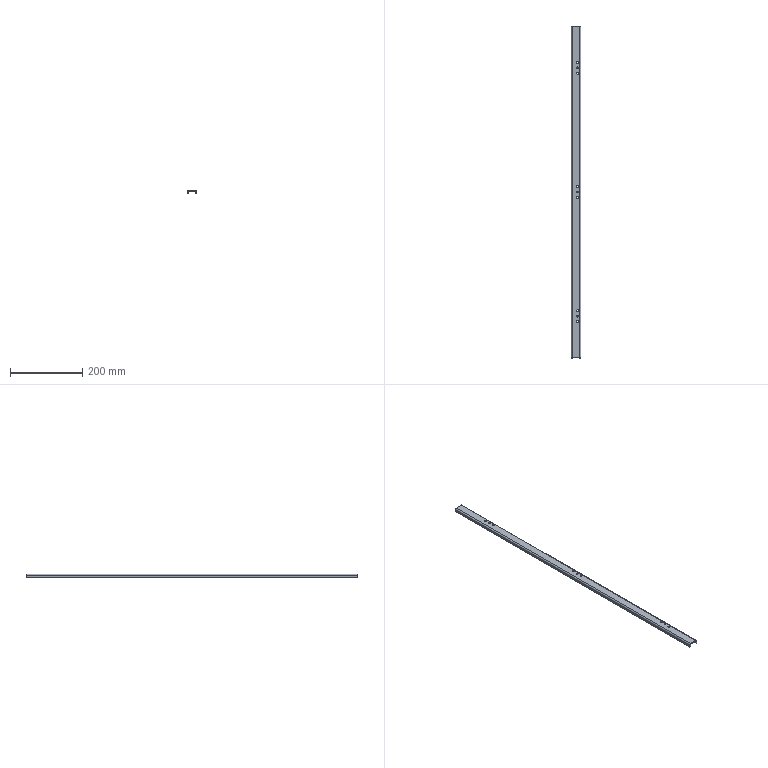Part | SolidWorks | features BaseBody 1 | 1 solid | 40 faces | box 27 x 919.8 x 10 mm | volume 107825 mm3 | cylinder 22 | plane 18 | commonest cylinder face diameters 5.2 x18 1 x2 7 x2
STEP:
#1=CARTESIAN_POINT('',(1.9,0.,-3.));
#2=VERTEX_POINT('',#1);
#3=CARTESIAN_POINT('',(1.9,0.,0.));
#4=VERTEX_POINT('',#3);
#5=CARTESIAN_POINT('',(1.9,0.,-3.));
#6=DIRECTION('',(0.,0.,1.));
#7=VECTOR('',#6,1000.);
#8=LINE('',#5,#7);
#9=EDGE_CURVE('',#2,#4,#8,.T.);
#10=ORIENTED_EDGE('',*,*,#9,.F.);
#11=CARTESIAN_POINT('',(7.1,0.,-3.));
#12=VERTEX_POINT('',#11);
#13=CARTESIAN_POINT('',(4.5,0.,-3.));
#14=DIRECTION('',(0.,0.,1.));
#15=DIRECTION('',(1.,0.,0.));
#16=AXIS2_PLACEMENT_3D('',#13,#14,#15);
#17=CIRCLE('',#16,2.6);
#18=EDGE_CURVE('',#12,#2,#17,.T.);
#19=ORIENTED_EDGE('',*,*,#18,.F.);
#20=CARTESIAN_POINT('',(7.1,0.,0.));
#21=VERTEX_POINT('',#20);
#22=CARTESIAN_POINT('',(7.1,0.,-3.));
#23=DIRECTION('',(0.,0.,1.));
#24=VECTOR('',#23,1000.);
#25=LINE('',#22,#24);
#26=EDGE_CURVE('',#12,#21,#25,.T.);
#27=ORIENTED_EDGE('',*,*,#26,.T.);
#28=CARTESIAN_POINT('',(4.5,0.,0.));
#29=DIRECTION('',(0.,0.,1.));
#30=DIRECTION('',(1.,0.,0.));
#31=AXIS2_PLACEMENT_3D('',#28,#29,#30);
#32=CIRCLE('',#31,2.6);
#33=EDGE_CURVE('',#21,#4,#32,.T.);
#34=ORIENTED_EDGE('',*,*,#33,.T.);
#35=EDGE_LOOP('',(#10,#19,#27,#34));
#36=FACE_OUTER_BOUND('',#35,.T.);
#37=CARTESIAN_POINT('',(4.5,0.,-3.));
#38=DIRECTION('',(0.,0.,1.));
#39=DIRECTION('',(1.,0.,0.));
#40=AXIS2_PLACEMENT_3D('',#37,#38,#39);
#41=CYLINDRICAL_SURFACE('',#40,2.6);
#42=ADVANCED_FACE('',(#36),#41,.F.);
#43=CARTESIAN_POINT('',(1.9,15.,-3.));
#44=VERTEX_POINT('',#43);
#45=CARTESIAN_POINT('',(1.9,15.,0.));
#46=VERTEX_POINT('',#45);
#47=CARTESIAN_POINT('',(1.9,15.,-3.));
#48=DIRECTION('',(0.,0.,1.));
#49=VECTOR('',#48,1000.);
#50=LINE('',#47,#49);
#51=EDGE_CURVE('',#44,#46,#50,.T.);
#52=ORIENTED_EDGE('',*,*,#51,.F.);
#53=CARTESIAN_POINT('',(7.1,15.,-3.));
#54=VERTEX_POINT('',#53);
#55=CARTESIAN_POINT('',(4.5,15.,-3.));
#56=DIRECTION('',(0.,0.,1.));
#57=DIRECTION('',(1.,0.,0.));
#58=AXIS2_PLACEMENT_3D('',#55,#56,#57);
#59=CIRCLE('',#58,2.6);
#60=EDGE_CURVE('',#54,#44,#59,.T.);
#61=ORIENTED_EDGE('',*,*,#60,.F.);
#62=CARTESIAN_POINT('',(7.1,15.,0.));
#63=VERTEX_POINT('',#62);
#64=CARTESIAN_POINT('',(7.1,15.,-3.));
#65=DIRECTION('',(0.,0.,1.));
#66=VECTOR('',#65,1000.);
#67=LINE('',#64,#66);
#68=EDGE_CURVE('',#54,#63,#67,.T.);
#69=ORIENTED_EDGE('',*,*,#68,.T.);
#70=CARTESIAN_POINT('',(4.5,15.,0.));
#71=DIRECTION('',(0.,0.,1.));
#72=DIRECTION('',(1.,0.,0.));
#73=AXIS2_PLACEMENT_3D('',#70,#71,#72);
#74=CIRCLE('',#73,2.6);
#75=EDGE_CURVE('',#63,#46,#74,.T.);
#76=ORIENTED_EDGE('',*,*,#75,.T.);
#77=EDGE_LOOP('',(#52,#61,#69,#76));
#78=FACE_OUTER_BOUND('',#77,.T.);
#79=CARTESIAN_POINT('',(4.5,15.,-3.));
#80=DIRECTION('',(0.,0.,1.));
#81=DIRECTION('',(1.,0.,0.));
#82=AXIS2_PLACEMENT_3D('',#79,#80,#81);
#83=CYLINDRICAL_SURFACE('',#82,2.6);
#84=ADVANCED_FACE('',(#78),#83,.F.);
#85=CARTESIAN_POINT('',(1.9,-15.,-3.));
#86=VERTEX_POINT('',#85);
#87=CARTESIAN_POINT('',(1.9,-15.,0.));
#88=VERTEX_POINT('',#87);
#89=CARTESIAN_POINT('',(1.9,-15.,-3.));
#90=DIRECTION('',(0.,0.,1.));
#91=VECTOR('',#90,1000.);
#92=LINE('',#89,#91);
#93=EDGE_CURVE('',#86,#88,#92,.T.);
#94=ORIENTED_EDGE('',*,*,#93,.F.);
#95=CARTESIAN_POINT('',(7.1,-15.,-3.));
#96=VERTEX_POINT('',#95);
#97=CARTESIAN_POINT('',(4.5,-15.,-3.));
#98=DIRECTION('',(0.,0.,1.));
#99=DIRECTION('',(1.,0.,0.));
#100=AXIS2_PLACEMENT_3D('',#97,#98,#99);
#101=CIRCLE('',#100,2.6);
#102=EDGE_CURVE('',#96,#86,#101,.T.);
#103=ORIENTED_EDGE('',*,*,#102,.F.);
#104=CARTESIAN_POINT('',(7.1,-15.,0.));
#105=VERTEX_POINT('',#104);
#106=CARTESIAN_POINT('',(7.1,-15.,-3.));
#107=DIRECTION('',(0.,0.,1.));
#108=VECTOR('',#107,1000.);
#109=LINE('',#106,#108);
#110=EDGE_CURVE('',#96,#105,#109,.T.);
#111=ORIENTED_EDGE('',*,*,#110,.T.);
#112=CARTESIAN_POINT('',(4.5,-15.,0.));
#113=DIRECTION('',(0.,0.,1.));
#114=DIRECTION('',(1.,0.,0.));
#115=AXIS2_PLACEMENT_3D('',#112,#113,#114);
#116=CIRCLE('',#115,2.6);
#117=EDGE_CURVE('',#105,#88,#116,.T.);
#118=ORIENTED_EDGE('',*,*,#117,.T.);
#119=EDGE_LOOP('',(#94,#103,#111,#118));
#120=FACE_OUTER_BOUND('',#119,.T.);
#121=CARTESIAN_POINT('',(4.5,-15.,-3.));
#122=DIRECTION('',(0.,0.,1.));
#123=DIRECTION('',(1.,0.,0.));
#124=AXIS2_PLACEMENT_3D('',#121,#122,#123);
#125=CYLINDRICAL_SURFACE('',#124,2.6);
#126=ADVANCED_FACE('',(#120),#125,.F.);
#127=CARTESIAN_POINT('',(1.9,-359.,-3.));
#128=VERTEX_POINT('',#127);
#129=CARTESIAN_POINT('',(1.9,-359.,0.));
#130=VERTEX_POINT('',#129);
#131=CARTESIAN_POINT('',(1.9,-359.,-3.));
#132=DIRECTION('',(0.,0.,1.));
#133=VECTOR('',#132,1000.);
#134=LINE('',#131,#133);
#135=EDGE_CURVE('',#128,#130,#134,.T.);
#136=ORIENTED_EDGE('',*,*,#135,.F.);
#137=CARTESIAN_POINT('',(7.1,-359.,-3.));
#138=VERTEX_POINT('',#137);
#139=CARTESIAN_POINT('',(4.5,-359.,-3.));
#140=DIRECTION('',(0.,0.,1.));
#141=DIRECTION('',(1.,0.,0.));
#142=AXIS2_PLACEMENT_3D('',#139,#140,#141);
#143=CIRCLE('',#142,2.6);
#144=EDGE_CURVE('',#138,#128,#143,.T.);
#145=ORIENTED_EDGE('',*,*,#144,.F.);
#146=CARTESIAN_POINT('',(7.1,-359.,0.));
#147=VERTEX_POINT('',#146);
#148=CARTESIAN_POINT('',(7.1,-359.,-3.));
#149=DIRECTION('',(0.,0.,1.));
#150=VECTOR('',#149,1000.);
#151=LINE('',#148,#150);
#152=EDGE_CURVE('',#138,#147,#151,.T.);
#153=ORIENTED_EDGE('',*,*,#152,.T.);
#154=CARTESIAN_POINT('',(4.5,-359.,0.));
#155=DIRECTION('',(0.,0.,1.));
#156=DIRECTION('',(1.,0.,0.));
#157=AXIS2_PLACEMENT_3D('',#154,#155,#156);
#158=CIRCLE('',#157,2.6);
#159=EDGE_CURVE('',#147,#130,#158,.T.);
#160=ORIENTED_EDGE('',*,*,#159,.T.);
#161=EDGE_LOOP('',(#136,#145,#153,#160));
#162=FACE_OUTER_BOUND('',#161,.T.);
#163=CARTESIAN_POINT('',(4.5,-359.,-3.));
#164=DIRECTION('',(0.,0.,1.));
#165=DIRECTION('',(1.,0.,0.));
#166=AXIS2_PLACEMENT_3D('',#163,#164,#165);
#167=CYLINDRICAL_SURFACE('',#166,2.6);
#168=ADVANCED_FACE('',(#162),#167,.F.);
#169=CARTESIAN_POINT('',(1.9,-344.,-3.));
#170=VERTEX_POINT('',#169);
#171=CARTESIAN_POINT('',(1.9,-344.,0.));
#172=VERTEX_POINT('',#171);
#173=CARTESIAN_POINT('',(1.9,-344.,-3.));
#174=DIRECTION('',(0.,0.,1.));
#175=VECTOR('',#174,1000.);
#176=LINE('',#173,#175);
#177=EDGE_CURVE('',#170,#172,#176,.T.);
#178=ORIENTED_EDGE('',*,*,#177,.F.);
#179=CARTESIAN_POINT('',(7.1,-344.,-3.));
#180=VERTEX_POINT('',#179);
#181=CARTESIAN_POINT('',(4.5,-344.,-3.));
#182=DIRECTION('',(0.,0.,1.));
#183=DIRECTION('',(1.,0.,0.));
#184=AXIS2_PLACEMENT_3D('',#181,#182,#183);
#185=CIRCLE('',#184,2.6);
#186=EDGE_CURVE('',#180,#170,#185,.T.);
#187=ORIENTED_EDGE('',*,*,#186,.F.);
#188=CARTESIAN_POINT('',(7.1,-344.,0.));
#189=VERTEX_POINT('',#188);
#190=CARTESIAN_POINT('',(7.1,-344.,-3.));
#191=DIRECTION('',(0.,0.,1.));
#192=VECTOR('',#191,1000.);
#193=LINE('',#190,#192);
#194=EDGE_CURVE('',#180,#189,#193,.T.);
#195=ORIENTED_EDGE('',*,*,#194,.T.);
#196=CARTESIAN_POINT('',(4.5,-344.,0.));
#197=DIRECTION('',(0.,0.,1.));
#198=DIRECTION('',(1.,0.,0.));
#199=AXIS2_PLACEMENT_3D('',#196,#197,#198);
#200=CIRCLE('',#199,2.6);
#201=EDGE_CURVE('',#189,#172,#200,.T.);
#202=ORIENTED_EDGE('',*,*,#201,.T.);
#203=EDGE_LOOP('',(#178,#187,#195,#202));
#204=FACE_OUTER_BOUND('',#203,.T.);
#205=CARTESIAN_POINT('',(4.5,-344.,-3.));
#206=DIRECTION('',(0.,0.,1.));
#207=DIRECTION('',(1.,0.,0.));
#208=AXIS2_PLACEMENT_3D('',#205,#206,#207);
#209=CYLINDRICAL_SURFACE('',#208,2.6);
#210=ADVANCED_FACE('',(#204),#209,.F.);
#211=CARTESIAN_POINT('',(1.9,-329.,-3.));
#212=VERTEX_POINT('',#211);
#213=CARTESIAN_POINT('',(1.9,-329.,0.));
#214=VERTEX_POINT('',#213);
#215=CARTESIAN_POINT('',(1.9,-329.,-3.));
#216=DIRECTION('',(0.,0.,1.));
#217=VECTOR('',#216,1000.);
#218=LINE('',#215,#217);
#219=EDGE_CURVE('',#212,#214,#218,.T.);
#220=ORIENTED_EDGE('',*,*,#219,.F.);
#221=CARTESIAN_POINT('',(7.1,-329.,-3.));
#222=VERTEX_POINT('',#221);
#223=CARTESIAN_POINT('',(4.5,-329.,-3.));
#224=DIRECTION('',(0.,0.,1.));
#225=DIRECTION('',(1.,0.,0.));
#226=AXIS2_PLACEMENT_3D('',#223,#224,#225);
#227=CIRCLE('',#226,2.6);
#228=EDGE_CURVE('',#222,#212,#227,.T.);
#229=ORIENTED_EDGE('',*,*,#228,.F.);
#230=CARTESIAN_POINT('',(7.1,-329.,0.));
#231=VERTEX_POINT('',#230);
#232=CARTESIAN_POINT('',(7.1,-329.,-3.));
#233=DIRECTION('',(0.,0.,1.));
#234=VECTOR('',#233,1000.);
#235=LINE('',#232,#234);
#236=EDGE_CURVE('',#222,#231,#235,.T.);
#237=ORIENTED_EDGE('',*,*,#236,.T.);
#238=CARTESIAN_POINT('',(4.5,-329.,0.));
#239=DIRECTION('',(0.,0.,1.));
#240=DIRECTION('',(1.,0.,0.));
#241=AXIS2_PLACEMENT_3D('',#238,#239,#240);
#242=CIRCLE('',#241,2.6);
#243=EDGE_CURVE('',#231,#214,#242,.T.);
#244=ORIENTED_EDGE('',*,*,#243,.T.);
#245=EDGE_LOOP('',(#220,#229,#237,#244));
#246=FACE_OUTER_BOUND('',#245,.T.);
#247=CARTESIAN_POINT('',(4.5,-329.,-3.));
#248=DIRECTION('',(0.,0.,1.));
#249=DIRECTION('',(1.,0.,0.));
#250=AXIS2_PLACEMENT_3D('',#247,#248,#249);
#251=CYLINDRICAL_SURFACE('',#250,2.6);
#252=ADVANCED_FACE('',(#246),#251,.F.);
#253=CARTESIAN_POINT('',(-10.5,459.9,-10.));
#254=VERTEX_POINT('',#253);
#255=CARTESIAN_POINT('',(-10.5,-459.9,-10.));
#256=VERTEX_POINT('',#255);
#257=CARTESIAN_POINT('',(-10.5,-459.9,-10.));
#258=DIRECTION('',(0.,-1.,0.));
#259=VECTOR('',#258,1000.);
#260=LINE('',#257,#259);
#261=EDGE_CURVE('',#254,#256,#260,.T.);
#262=ORIENTED_EDGE('',*,*,#261,.T.);
#263=CARTESIAN_POINT('',(-13.5,-459.9,-10.));
#264=VERTEX_POINT('',#263);
#265=CARTESIAN_POINT('',(-13.5,-459.9,-10.));
#266=DIRECTION('',(1.,0.,0.));
#267=VECTOR('',#266,1000.);
#268=LINE('',#265,#267);
#269=EDGE_CURVE('',#264,#256,#268,.T.);
#270=ORIENTED_EDGE('',*,*,#269,.F.);
#271=CARTESIAN_POINT('',(-13.5,459.9,-10.));
#272=VERTEX_POINT('',#271);
#273=CARTESIAN_POINT('',(-13.5,0.,-10.));
#274=DIRECTION('',(0.,-1.,0.));
#275=VECTOR('',#274,1000.);
#276=LINE('',#273,#275);
#277=EDGE_CURVE('',#272,#264,#276,.T.);
#278=ORIENTED_EDGE('',*,*,#277,.F.);
#279=CARTESIAN_POINT('',(-13.5,459.9,-10.));
#280=DIRECTION('',(1.,0.,0.));
#281=VECTOR('',#280,1000.);
#282=LINE('',#279,#281);
#283=EDGE_CURVE('',#272,#254,#282,.T.);
#284=ORIENTED_EDGE('',*,*,#283,.T.);
#285=EDGE_LOOP('',(#262,#270,#278,#284));
#286=FACE_OUTER_BOUND('',#285,.T.);
#287=CARTESIAN_POINT('',(-13.5,-459.9,-10.));
#288=DIRECTION('',(0.,0.,1.));
#289=DIRECTION('',(1.,0.,0.));
#290=AXIS2_PLACEMENT_3D('',#287,#288,#289);
#291=PLANE('',#290);
#292=ADVANCED_FACE('',(#286),#291,.F.);
#293=CARTESIAN_POINT('',(-10.5,459.9,-3.5));
#294=VERTEX_POINT('',#293);
#295=CARTESIAN_POINT('',(-10.5,459.9,-10.));
#296=DIRECTION('',(0.,0.,-1.));
#297=VECTOR('',#296,1000.);
#298=LINE('',#295,#297);
#299=EDGE_CURVE('',#294,#254,#298,.T.);
#300=ORIENTED_EDGE('',*,*,#299,.F.);
#301=CARTESIAN_POINT('',(-10.5,-459.9,-3.5));
#302=VERTEX_POINT('',#301);
#303=CARTESIAN_POINT('',(-10.5,-459.9,-3.5));
#304=DIRECTION('',(0.,1.,0.));
#305=VECTOR('',#304,1000.);
#306=LINE('',#303,#305);
#307=EDGE_CURVE('',#302,#294,#306,.T.);
#308=ORIENTED_EDGE('',*,*,#307,.F.);
#309=CARTESIAN_POINT('',(-10.5,-459.9,-3.));
#310=DIRECTION('',(0.,0.,1.));
#311=VECTOR('',#310,1000.);
#312=LINE('',#309,#311);
#313=EDGE_CURVE('',#256,#302,#312,.T.);
#314=ORIENTED_EDGE('',*,*,#313,.F.);
#315=ORIENTED_EDGE('',*,*,#261,.F.);
#316=EDGE_LOOP('',(#300,#308,#314,#315));
#317=FACE_OUTER_BOUND('',#316,.T.);
#318=CARTESIAN_POINT('',(-10.5,0.,0.));
#319=DIRECTION('',(1.,0.,0.));
#320=DIRECTION('',(0.,0.,-1.));
#321=AXIS2_PLACEMENT_3D('',#318,#319,#320);
#322=PLANE('',#321);
#323=ADVANCED_FACE('',(#317),#322,.T.);
#324=CARTESIAN_POINT('',(-13.5,459.9,-3.5));
#325=VERTEX_POINT('',#324);
#326=CARTESIAN_POINT('',(-13.5,-459.9,-3.5));
#327=VERTEX_POINT('',#326);
#328=CARTESIAN_POINT('',(-13.5,-459.9,-3.5));
#329=DIRECTION('',(0.,-1.,0.));
#330=VECTOR('',#329,1000.);
#331=LINE('',#328,#330);
#332=EDGE_CURVE('',#325,#327,#331,.T.);
#333=ORIENTED_EDGE('',*,*,#332,.F.);
#334=CARTESIAN_POINT('',(-13.5,459.9,0.));
#335=DIRECTION('',(0.,0.,-1.));
#336=VECTOR('',#335,1000.);
#337=LINE('',#334,#336);
#338=EDGE_CURVE('',#325,#272,#337,.T.);
#339=ORIENTED_EDGE('',*,*,#338,.T.);
#340=ORIENTED_EDGE('',*,*,#277,.T.);
#341=CARTESIAN_POINT('',(-13.5,-459.9,0.));
#342=DIRECTION('',(0.,0.,1.));
#343=VECTOR('',#342,1000.);
#344=LINE('',#341,#343);
#345=EDGE_CURVE('',#264,#327,#344,.T.);
#346=ORIENTED_EDGE('',*,*,#345,.T.);
#347=EDGE_LOOP('',(#333,#339,#340,#346));
#348=FACE_OUTER_BOUND('',#347,.T.);
#349=CARTESIAN_POINT('',(-13.5,0.,0.));
#350=DIRECTION('',(1.,0.,0.));
#351=DIRECTION('',(0.,0.,-1.));
#352=AXIS2_PLACEMENT_3D('',#349,#350,#351);
#353=PLANE('',#352);
#354=ADVANCED_FACE('',(#348),#353,.F.);
#355=CARTESIAN_POINT('',(-13.5,-459.9,-3.5));
#356=DIRECTION('',(-1.,0.,0.));
#357=VECTOR('',#356,1000.);
#358=LINE('',#355,#357);
#359=EDGE_CURVE('',#302,#327,#358,.T.);
#360=ORIENTED_EDGE('',*,*,#359,.T.);
#361=ORIENTED_EDGE('',*,*,#345,.F.);
#362=ORIENTED_EDGE('',*,*,#269,.T.);
#363=ORIENTED_EDGE('',*,*,#313,.T.);
#364=EDGE_LOOP('',(#360,#361,#362,#363));
#365=FACE_OUTER_BOUND('',#364,.T.);
#366=CARTESIAN_POINT('',(-13.5,-459.9,-3.));
#367=DIRECTION('',(0.,1.,0.));
#368=DIRECTION('',(1.,0.,0.));
#369=AXIS2_PLACEMENT_3D('',#366,#367,#368);
#370=PLANE('',#369);
#371=ADVANCED_FACE('',(#365),#370,.F.);
#372=CARTESIAN_POINT('',(-10.5,459.9,-3.5));
#373=DIRECTION('',(-1.,0.,0.));
#374=VECTOR('',#373,1000.);
#375=LINE('',#372,#374);
#376=EDGE_CURVE('',#294,#325,#375,.T.);
#377=ORIENTED_EDGE('',*,*,#376,.F.);
#378=ORIENTED_EDGE('',*,*,#299,.T.);
#379=ORIENTED_EDGE('',*,*,#283,.F.);
#380=ORIENTED_EDGE('',*,*,#338,.F.);
#381=EDGE_LOOP('',(#377,#378,#379,#380));
#382=FACE_OUTER_BOUND('',#381,.T.);
#383=CARTESIAN_POINT('',(-13.5,459.9,-10.));
#384=DIRECTION('',(0.,-1.,0.));
#385=DIRECTION('',(0.,0.,-1.));
#386=AXIS2_PLACEMENT_3D('',#383,#384,#385);
#387=PLANE('',#386);
#388=ADVANCED_FACE('',(#382),#387,.F.);
#389=CARTESIAN_POINT('',(-10.,459.9,-3.));
#390=VERTEX_POINT('',#389);
#391=CARTESIAN_POINT('',(-10.,-459.9,-3.));
#392=VERTEX_POINT('',#391);
#393=CARTESIAN_POINT('',(-10.,459.9,-3.));
#394=DIRECTION('',(0.,-1.,0.));
#395=VECTOR('',#394,1000.);
#396=LINE('',#393,#395);
#397=EDGE_CURVE('',#390,#392,#396,.T.);
#398=ORIENTED_EDGE('',*,*,#397,.T.);
#399=CARTESIAN_POINT('',(-10.,-459.9,-3.5));
#400=DIRECTION('',(0.,-1.,0.));
#401=DIRECTION('',(0.,0.,1.));
#402=AXIS2_PLACEMENT_3D('',#399,#400,#401);
#403=CIRCLE('',#402,0.5);
#404=EDGE_CURVE('',#392,#302,#403,.T.);
#405=ORIENTED_EDGE('',*,*,#404,.T.);
#406=ORIENTED_EDGE('',*,*,#307,.T.);
#407=CARTESIAN_POINT('',(-10.,459.9,-3.5));
#408=DIRECTION('',(0.,1.,0.));
#409=DIRECTION('',(0.,0.,1.));
#410=AXIS2_PLACEMENT_3D('',#407,#408,#409);
#411=CIRCLE('',#410,0.5);
#412=EDGE_CURVE('',#294,#390,#411,.T.);
#413=ORIENTED_EDGE('',*,*,#412,.T.);
#414=EDGE_LOOP('',(#398,#405,#406,#413));
#415=FACE_OUTER_BOUND('',#414,.T.);
#416=CARTESIAN_POINT('',(-10.,459.9,-3.5));
#417=DIRECTION('',(0.,1.,0.));
#418=DIRECTION('',(-1.,0.,0.));
#419=AXIS2_PLACEMENT_3D('',#416,#417,#418);
#420=CYLINDRICAL_SURFACE('',#419,0.5);
#421=ADVANCED_FACE('',(#415),#420,.F.);
#422=CARTESIAN_POINT('',(-10.,459.9,0.));
#423=VERTEX_POINT('',#422);
#424=CARTESIAN_POINT('',(-10.,-459.9,0.));
#425=VERTEX_POINT('',#424);
#426=CARTESIAN_POINT('',(-10.,459.9,0.));
#427=DIRECTION('',(0.,-1.,0.));
#428=VECTOR('',#427,1000.);
#429=LINE('',#426,#428);
#430=EDGE_CURVE('',#423,#425,#429,.T.);
#431=ORIENTED_EDGE('',*,*,#430,.F.);
#432=CARTESIAN_POINT('',(-10.,459.9,-3.5));
#433=DIRECTION('',(0.,1.,0.));
#434=DIRECTION('',(0.,0.,1.));
#435=AXIS2_PLACEMENT_3D('',#432,#433,#434);
#436=CIRCLE('',#435,3.5);
#437=EDGE_CURVE('',#325,#423,#436,.T.);
#438=ORIENTED_EDGE('',*,*,#437,.F.);
#439=ORIENTED_EDGE('',*,*,#332,.T.);
#440=CARTESIAN_POINT('',(-10.,-459.9,-3.5));
#441=DIRECTION('',(0.,-1.,0.));
#442=DIRECTION('',(0.,0.,1.));
#443=AXIS2_PLACEMENT_3D('',#440,#441,#442);
#444=CIRCLE('',#443,3.5);
#445=EDGE_CURVE('',#425,#327,#444,.T.);
#446=ORIENTED_EDGE('',*,*,#445,.F.);
#447=EDGE_LOOP('',(#431,#438,#439,#446));
#448=FACE_OUTER_BOUND('',#447,.T.);
#449=CARTESIAN_POINT('',(-10.,459.9,-3.5));
#450=DIRECTION('',(0.,1.,0.));
#451=DIRECTION('',(-1.,0.,0.));
#452=AXIS2_PLACEMENT_3D('',#449,#450,#451);
#453=CYLINDRICAL_SURFACE('',#452,3.5);
#454=ADVANCED_FACE('',(#448),#453,.T.);
#455=ORIENTED_EDGE('',*,*,#412,.F.);
#456=ORIENTED_EDGE('',*,*,#376,.T.);
#457=ORIENTED_EDGE('',*,*,#437,.T.);
#458=CARTESIAN_POINT('',(-10.,459.9,-3.));
#459=DIRECTION('',(0.,0.,1.));
#460=VECTOR('',#459,1000.);
#461=LINE('',#458,#460);
#462=EDGE_CURVE('',#390,#423,#461,.T.);
#463=ORIENTED_EDGE('',*,*,#462,.F.);
#464=EDGE_LOOP('',(#455,#456,#457,#463));
#465=FACE_OUTER_BOUND('',#464,.T.);
#466=CARTESIAN_POINT('',(-10.,459.9,-3.5));
#467=DIRECTION('',(0.,-1.,0.));
#468=DIRECTION('',(0.,0.,-1.));
#469=AXIS2_PLACEMENT_3D('',#466,#467,#468);
#470=PLANE('',#469);
#471=ADVANCED_FACE('',(#465),#470,.F.);
#472=ORIENTED_EDGE('',*,*,#359,.F.);
#473=ORIENTED_EDGE('',*,*,#404,.F.);
#474=CARTESIAN_POINT('',(-10.,-459.9,-3.));
#475=DIRECTION('',(0.,0.,1.));
#476=VECTOR('',#475,1000.);
#477=LINE('',#474,#476);
#478=EDGE_CURVE('',#392,#425,#477,.T.);
#479=ORIENTED_EDGE('',*,*,#478,.T.);
#480=ORIENTED_EDGE('',*,*,#445,.T.);
#481=EDGE_LOOP('',(#472,#473,#479,#480));
#482=FACE_OUTER_BOUND('',#481,.T.);
#483=CARTESIAN_POINT('',(-10.,-459.9,-3.5));
#484=DIRECTION('',(0.,-1.,0.));
#485=DIRECTION('',(0.,0.,-1.));
#486=AXIS2_PLACEMENT_3D('',#483,#484,#485);
#487=PLANE('',#486);
#488=ADVANCED_FACE('',(#482),#487,.T.);
#489=CARTESIAN_POINT('',(10.5,-459.9,-10.));
#490=VERTEX_POINT('',#489);
#491=CARTESIAN_POINT('',(10.5,459.9,-10.));
#492=VERTEX_POINT('',#491);
#493=CARTESIAN_POINT('',(10.5,459.9,-10.));
#494=DIRECTION('',(0.,1.,0.));
#495=VECTOR('',#494,1000.);
#496=LINE('',#493,#495);
#497=EDGE_CURVE('',#490,#492,#496,.T.);
#498=ORIENTED_EDGE('',*,*,#497,.T.);
#499=CARTESIAN_POINT('',(13.5,459.9,-10.));
#500=VERTEX_POINT('',#499);
#501=CARTESIAN_POINT('',(13.5,459.9,-10.));
#502=DIRECTION('',(-1.,0.,0.));
#503=VECTOR('',#502,1000.);
#504=LINE('',#501,#503);
#505=EDGE_CURVE('',#500,#492,#504,.T.);
#506=ORIENTED_EDGE('',*,*,#505,.F.);
#507=CARTESIAN_POINT('',(13.5,-459.9,-10.));
#508=VERTEX_POINT('',#507);
#509=CARTESIAN_POINT('',(13.5,0.,-10.));
#510=DIRECTION('',(0.,1.,0.));
#511=VECTOR('',#510,1000.);
#512=LINE('',#509,#511);
#513=EDGE_CURVE('',#508,#500,#512,.T.);
#514=ORIENTED_EDGE('',*,*,#513,.F.);
#515=CARTESIAN_POINT('',(13.5,-459.9,-10.));
#516=DIRECTION('',(-1.,0.,0.));
#517=VECTOR('',#516,1000.);
#518=LINE('',#515,#517);
#519=EDGE_CURVE('',#508,#490,#518,.T.);
#520=ORIENTED_EDGE('',*,*,#519,.T.);
#521=EDGE_LOOP('',(#498,#506,#514,#520));
#522=FACE_OUTER_BOUND('',#521,.T.);
#523=CARTESIAN_POINT('',(13.5,459.9,-10.));
#524=DIRECTION('',(0.,0.,1.));
#525=DIRECTION('',(1.,0.,0.));
#526=AXIS2_PLACEMENT_3D('',#523,#524,#525);
#527=PLANE('',#526);
#528=ADVANCED_FACE('',(#522),#527,.F.);
#529=CARTESIAN_POINT('',(10.5,-459.9,-3.5));
#530=VERTEX_POINT('',#529);
#531=CARTESIAN_POINT('',(10.5,-459.9,-10.));
#532=DIRECTION('',(0.,0.,-1.));
#533=VECTOR('',#532,1000.);
#534=LINE('',#531,#533);
#535=EDGE_CURVE('',#530,#490,#534,.T.);
#536=ORIENTED_EDGE('',*,*,#535,.F.);
#537=CARTESIAN_POINT('',(10.5,459.9,-3.5));
#538=VERTEX_POINT('',#537);
#539=CARTESIAN_POINT('',(10.5,459.9,-3.5));
#540=DIRECTION('',(0.,-1.,0.));
#541=VECTOR('',#540,1000.);
#542=LINE('',#539,#541);
#543=EDGE_CURVE('',#538,#530,#542,.T.);
#544=ORIENTED_EDGE('',*,*,#543,.F.);
#545=CARTESIAN_POINT('',(10.5,459.9,-3.));
#546=DIRECTION('',(0.,0.,1.));
#547=VECTOR('',#546,1000.);
#548=LINE('',#545,#547);
#549=EDGE_CURVE('',#492,#538,#548,.T.);
#550=ORIENTED_EDGE('',*,*,#549,.F.);
#551=ORIENTED_EDGE('',*,*,#497,.F.);
#552=EDGE_LOOP('',(#536,#544,#550,#551));
#553=FACE_OUTER_BOUND('',#552,.T.);
#554=CARTESIAN_POINT('',(10.5,0.,0.));
#555=DIRECTION('',(-1.,0.,0.));
#556=DIRECTION('',(0.,0.,1.));
#557=AXIS2_PLACEMENT_3D('',#554,#555,#556);
#558=PLANE('',#557);
#559=ADVANCED_FACE('',(#553),#558,.T.);
#560=CARTESIAN_POINT('',(13.5,-459.9,-3.5));
#561=VERTEX_POINT('',#560);
#562=CARTESIAN_POINT('',(13.5,459.9,-3.5));
#563=VERTEX_POINT('',#562);
#564=CARTESIAN_POINT('',(13.5,459.9,-3.5));
#565=DIRECTION('',(0.,1.,0.));
#566=VECTOR('',#565,1000.);
#567=LINE('',#564,#566);
#568=EDGE_CURVE('',#561,#563,#567,.T.);
#569=ORIENTED_EDGE('',*,*,#568,.F.);
#570=CARTESIAN_POINT('',(13.5,-459.9,0.));
#571=DIRECTION('',(0.,0.,-1.));
#572=VECTOR('',#571,1000.);
#573=LINE('',#570,#572);
#574=EDGE_CURVE('',#561,#508,#573,.T.);
#575=ORIENTED_EDGE('',*,*,#574,.T.);
#576=ORIENTED_EDGE('',*,*,#513,.T.);
#577=CARTESIAN_POINT('',(13.5,459.9,0.));
#578=DIRECTION('',(0.,0.,1.));
#579=VECTOR('',#578,1000.);
#580=LINE('',#577,#579);
#581=EDGE_CURVE('',#500,#563,#580,.T.);
#582=ORIENTED_EDGE('',*,*,#581,.T.);
#583=EDGE_LOOP('',(#569,#575,#576,#582));
#584=FACE_OUTER_BOUND('',#583,.T.);
#585=CARTESIAN_POINT('',(13.5,0.,0.));
#586=DIRECTION('',(-1.,0.,0.));
#587=DIRECTION('',(0.,0.,1.));
#588=AXIS2_PLACEMENT_3D('',#585,#586,#587);
#589=PLANE('',#588);
#590=ADVANCED_FACE('',(#584),#589,.F.);
#591=CARTESIAN_POINT('',(13.5,459.9,-3.5));
#592=DIRECTION('',(1.,0.,0.));
#593=VECTOR('',#592,1000.);
#594=LINE('',#591,#593);
#595=EDGE_CURVE('',#538,#563,#594,.T.);
#596=ORIENTED_EDGE('',*,*,#595,.T.);
#597=ORIENTED_EDGE('',*,*,#581,.F.);
#598=ORIENTED_EDGE('',*,*,#505,.T.);
#599=ORIENTED_EDGE('',*,*,#549,.T.);
#600=EDGE_LOOP('',(#596,#597,#598,#599));
#601=FACE_OUTER_BOUND('',#600,.T.);
#602=CARTESIAN_POINT('',(13.5,459.9,-3.));
#603=DIRECTION('',(0.,-1.,0.));
#604=DIRECTION('',(0.,0.,-1.));
#605=AXIS2_PLACEMENT_3D('',#602,#603,#604);
#606=PLANE('',#605);
#607=ADVANCED_FACE('',(#601),#606,.F.);
#608=CARTESIAN_POINT('',(10.5,-459.9,-3.5));
#609=DIRECTION('',(1.,0.,0.));
#610=VECTOR('',#609,1000.);
#611=LINE('',#608,#610);
#612=EDGE_CURVE('',#530,#561,#611,.T.);
#613=ORIENTED_EDGE('',*,*,#612,.F.);
#614=ORIENTED_EDGE('',*,*,#535,.T.);
#615=ORIENTED_EDGE('',*,*,#519,.F.);
#616=ORIENTED_EDGE('',*,*,#574,.F.);
#617=EDGE_LOOP('',(#613,#614,#615,#616));
#618=FACE_OUTER_BOUND('',#617,.T.);
#619=CARTESIAN_POINT('',(13.5,-459.9,-10.));
#620=DIRECTION('',(0.,1.,0.));
#621=DIRECTION('',(1.,0.,0.));
#622=AXIS2_PLACEMENT_3D('',#619,#620,#621);
#623=PLANE('',#622);
#624=ADVANCED_FACE('',(#618),#623,.F.);
#625=CARTESIAN_POINT('',(10.,-459.9,-3.));
#626=VERTEX_POINT('',#625);
#627=CARTESIAN_POINT('',(10.,459.9,-3.));
#628=VERTEX_POINT('',#627);
#629=CARTESIAN_POINT('',(10.,-459.9,-3.));
#630=DIRECTION('',(0.,1.,0.));
#631=VECTOR('',#630,1000.);
#632=LINE('',#629,#631);
#633=EDGE_CURVE('',#626,#628,#632,.T.);
#634=ORIENTED_EDGE('',*,*,#633,.T.);
#635=CARTESIAN_POINT('',(10.,459.9,-3.5));
#636=DIRECTION('',(0.,1.,0.));
#637=DIRECTION('',(0.,0.,-1.));
#638=AXIS2_PLACEMENT_3D('',#635,#636,#637);
#639=CIRCLE('',#638,0.5);
#640=EDGE_CURVE('',#628,#538,#639,.T.);
#641=ORIENTED_EDGE('',*,*,#640,.T.);
#642=ORIENTED_EDGE('',*,*,#543,.T.);
#643=CARTESIAN_POINT('',(10.,-459.9,-3.5));
#644=DIRECTION('',(0.,-1.,0.));
#645=DIRECTION('',(0.,0.,-1.));
#646=AXIS2_PLACEMENT_3D('',#643,#644,#645);
#647=CIRCLE('',#646,0.5);
#648=EDGE_CURVE('',#530,#626,#647,.T.);
#649=ORIENTED_EDGE('',*,*,#648,.T.);
#650=EDGE_LOOP('',(#634,#641,#642,#649));
#651=FACE_OUTER_BOUND('',#650,.T.);
#652=CARTESIAN_POINT('',(10.,-459.9,-3.5));
#653=DIRECTION('',(0.,-1.,0.));
#654=DIRECTION('',(1.,0.,0.));
#655=AXIS2_PLACEMENT_3D('',#652,#653,#654);
#656=CYLINDRICAL_SURFACE('',#655,0.5);
#657=ADVANCED_FACE('',(#651),#656,.F.);
#658=CARTESIAN_POINT('',(10.,-459.9,0.));
#659=VERTEX_POINT('',#658);
#660=CARTESIAN_POINT('',(10.,459.9,0.));
#661=VERTEX_POINT('',#660);
#662=CARTESIAN_POINT('',(10.,-459.9,0.));
#663=DIRECTION('',(0.,1.,0.));
#664=VECTOR('',#663,1000.);
#665=LINE('',#662,#664);
#666=EDGE_CURVE('',#659,#661,#665,.T.);
#667=ORIENTED_EDGE('',*,*,#666,.F.);
#668=CARTESIAN_POINT('',(10.,-459.9,-3.5));
#669=DIRECTION('',(0.,-1.,0.));
#670=DIRECTION('',(0.,0.,-1.));
#671=AXIS2_PLACEMENT_3D('',#668,#669,#670);
#672=CIRCLE('',#671,3.5);
#673=EDGE_CURVE('',#561,#659,#672,.T.);
#674=ORIENTED_EDGE('',*,*,#673,.F.);
#675=ORIENTED_EDGE('',*,*,#568,.T.);
#676=CARTESIAN_POINT('',(10.,459.9,-3.5));
#677=DIRECTION('',(0.,1.,0.));
#678=DIRECTION('',(0.,0.,-1.));
#679=AXIS2_PLACEMENT_3D('',#676,#677,#678);
#680=CIRCLE('',#679,3.5);
#681=EDGE_CURVE('',#661,#563,#680,.T.);
#682=ORIENTED_EDGE('',*,*,#681,.F.);
#683=EDGE_LOOP('',(#667,#674,#675,#682));
#684=FACE_OUTER_BOUND('',#683,.T.);
#685=CARTESIAN_POINT('',(10.,-459.9,-3.5));
#686=DIRECTION('',(0.,-1.,0.));
#687=DIRECTION('',(1.,0.,0.));
#688=AXIS2_PLACEMENT_3D('',#685,#686,#687);
#689=CYLINDRICAL_SURFACE('',#688,3.5);
#690=ADVANCED_FACE('',(#684),#689,.T.);
#691=ORIENTED_EDGE('',*,*,#648,.F.);
#692=ORIENTED_EDGE('',*,*,#612,.T.);
#693=ORIENTED_EDGE('',*,*,#673,.T.);
#694=CARTESIAN_POINT('',(10.,-459.9,-3.));
#695=DIRECTION('',(0.,0.,1.));
#696=VECTOR('',#695,1000.);
#697=LINE('',#694,#696);
#698=EDGE_CURVE('',#626,#659,#697,.T.);
#699=ORIENTED_EDGE('',*,*,#698,.F.);
#700=EDGE_LOOP('',(#691,#692,#693,#699));
#701=FACE_OUTER_BOUND('',#700,.T.);
#702=CARTESIAN_POINT('',(10.,-459.9,-3.5));
#703=DIRECTION('',(0.,1.,0.));
#704=DIRECTION('',(1.,0.,0.));
#705=AXIS2_PLACEMENT_3D('',#702,#703,#704);
#706=PLANE('',#705);
#707=ADVANCED_FACE('',(#701),#706,.F.);
#708=ORIENTED_EDGE('',*,*,#595,.F.);
#709=ORIENTED_EDGE('',*,*,#640,.F.);
#710=CARTESIAN_POINT('',(10.,459.9,-3.));
#711=DIRECTION('',(0.,0.,1.));
#712=VECTOR('',#711,1000.);
#713=LINE('',#710,#712);
#714=EDGE_CURVE('',#628,#661,#713,.T.);
#715=ORIENTED_EDGE('',*,*,#714,.T.);
#716=ORIENTED_EDGE('',*,*,#681,.T.);
#717=EDGE_LOOP('',(#708,#709,#715,#716));
#718=FACE_OUTER_BOUND('',#717,.T.);
#719=CARTESIAN_POINT('',(10.,459.9,-3.5));
#720=DIRECTION('',(0.,1.,0.));
#721=DIRECTION('',(1.,0.,0.));
#722=AXIS2_PLACEMENT_3D('',#719,#720,#721);
#723=PLANE('',#722);
#724=ADVANCED_FACE('',(#718),#723,.T.);
#725=ORIENTED_EDGE('',*,*,#478,.F.);
#726=CARTESIAN_POINT('',(13.5,-459.9,-3.));
#727=DIRECTION('',(1.,0.,0.));
#728=VECTOR('',#727,1000.);
#729=LINE('',#726,#728);
#730=EDGE_CURVE('',#392,#626,#729,.T.);
#731=ORIENTED_EDGE('',*,*,#730,.T.);
#732=ORIENTED_EDGE('',*,*,#698,.T.);
#733=CARTESIAN_POINT('',(13.5,-459.9,0.));
#734=DIRECTION('',(1.,0.,0.));
#735=VECTOR('',#734,1000.);
#736=LINE('',#733,#735);
#737=EDGE_CURVE('',#425,#659,#736,.T.);
#738=ORIENTED_EDGE('',*,*,#737,.F.);
#739=EDGE_LOOP('',(#725,#731,#732,#738));
#740=FACE_OUTER_BOUND('',#739,.T.);
#741=CARTESIAN_POINT('',(13.5,-459.9,-3.));
#742=DIRECTION('',(0.,-1.,0.));
#743=DIRECTION('',(0.,0.,-1.));
#744=AXIS2_PLACEMENT_3D('',#741,#742,#743);
#745=PLANE('',#744);
#746=ADVANCED_FACE('',(#740),#745,.T.);
#747=CARTESIAN_POINT('',(13.5,459.9,-3.));
#748=DIRECTION('',(-1.,0.,0.));
#749=VECTOR('',#748,1000.);
#750=LINE('',#747,#749);
#751=EDGE_CURVE('',#628,#390,#750,.T.);
#752=ORIENTED_EDGE('',*,*,#751,.T.);
#753=ORIENTED_EDGE('',*,*,#462,.T.);
#754=CARTESIAN_POINT('',(13.5,459.9,0.));
#755=DIRECTION('',(-1.,0.,0.));
#756=VECTOR('',#755,1000.);
#757=LINE('',#754,#756);
#758=EDGE_CURVE('',#661,#423,#757,.T.);
#759=ORIENTED_EDGE('',*,*,#758,.F.);
#760=ORIENTED_EDGE('',*,*,#714,.F.);
#761=EDGE_LOOP('',(#752,#753,#759,#760));
#762=FACE_OUTER_BOUND('',#761,.T.);
#763=CARTESIAN_POINT('',(13.5,459.9,-3.));
#764=DIRECTION('',(0.,1.,0.));
#765=DIRECTION('',(1.,0.,0.));
#766=AXIS2_PLACEMENT_3D('',#763,#764,#765);
#767=PLANE('',#766);
#768=ADVANCED_FACE('',(#762),#767,.T.);
#769=CARTESIAN_POINT('',(7.1,344.,0.));
#770=VERTEX_POINT('',#769);
#771=CARTESIAN_POINT('',(1.9,344.,0.));
#772=VERTEX_POINT('',#771);
#773=CARTESIAN_POINT('',(4.5,344.,0.));
#774=DIRECTION('',(0.,0.,1.));
#775=DIRECTION('',(1.,0.,0.));
#776=AXIS2_PLACEMENT_3D('',#773,#774,#775);
#777=CIRCLE('',#776,2.6);
#778=EDGE_CURVE('',#770,#772,#777,.T.);
#779=ORIENTED_EDGE('',*,*,#778,.F.);
#780=CARTESIAN_POINT('',(4.5,344.,0.));
#781=DIRECTION('',(0.,0.,1.));
#782=DIRECTION('',(1.,0.,0.));
#783=AXIS2_PLACEMENT_3D('',#780,#781,#782);
#784=CIRCLE('',#783,2.6);
#785=EDGE_CURVE('',#772,#770,#784,.T.);
#786=ORIENTED_EDGE('',*,*,#785,.F.);
#787=EDGE_LOOP('',(#779,#786));
#788=FACE_BOUND('',#787,.T.);
#789=CARTESIAN_POINT('',(7.1,359.,0.));
#790=VERTEX_POINT('',#789);
#791=CARTESIAN_POINT('',(1.9,359.,0.));
#792=VERTEX_POINT('',#791);
#793=CARTESIAN_POINT('',(4.5,359.,0.));
#794=DIRECTION('',(0.,0.,1.));
#795=DIRECTION('',(1.,0.,0.));
#796=AXIS2_PLACEMENT_3D('',#793,#794,#795);
#797=CIRCLE('',#796,2.6);
#798=EDGE_CURVE('',#790,#792,#797,.T.);
#799=ORIENTED_EDGE('',*,*,#798,.F.);
#800=CARTESIAN_POINT('',(4.5,359.,0.));
#801=DIRECTION('',(0.,0.,1.));
#802=DIRECTION('',(1.,0.,0.));
#803=AXIS2_PLACEMENT_3D('',#800,#801,#802);
#804=CIRCLE('',#803,2.6);
#805=EDGE_CURVE('',#792,#790,#804,.T.);
#806=ORIENTED_EDGE('',*,*,#805,.F.);
#807=EDGE_LOOP('',(#799,#806));
#808=FACE_BOUND('',#807,.T.);
#809=CARTESIAN_POINT('',(7.1,329.,0.));
#810=VERTEX_POINT('',#809);
#811=CARTESIAN_POINT('',(1.9,329.,0.));
#812=VERTEX_POINT('',#811);
#813=CARTESIAN_POINT('',(4.5,329.,0.));
#814=DIRECTION('',(0.,0.,1.));
#815=DIRECTION('',(1.,0.,0.));
#816=AXIS2_PLACEMENT_3D('',#813,#814,#815);
#817=CIRCLE('',#816,2.6);
#818=EDGE_CURVE('',#810,#812,#817,.T.);
#819=ORIENTED_EDGE('',*,*,#818,.F.);
#820=CARTESIAN_POINT('',(4.5,329.,0.));
#821=DIRECTION('',(0.,0.,1.));
#822=DIRECTION('',(1.,0.,0.));
#823=AXIS2_PLACEMENT_3D('',#820,#821,#822);
#824=CIRCLE('',#823,2.6);
#825=EDGE_CURVE('',#812,#810,#824,.T.);
#826=ORIENTED_EDGE('',*,*,#825,.F.);
#827=EDGE_LOOP('',(#819,#826));
#828=FACE_BOUND('',#827,.T.);
#829=ORIENTED_EDGE('',*,*,#243,.F.);
#830=CARTESIAN_POINT('',(4.5,-329.,0.));
#831=DIRECTION('',(0.,0.,1.));
#832=DIRECTION('',(1.,0.,0.));
#833=AXIS2_PLACEMENT_3D('',#830,#831,#832);
#834=CIRCLE('',#833,2.6);
#835=EDGE_CURVE('',#214,#231,#834,.T.);
#836=ORIENTED_EDGE('',*,*,#835,.F.);
#837=EDGE_LOOP('',(#829,#836));
#838=FACE_BOUND('',#837,.T.);
#839=ORIENTED_EDGE('',*,*,#201,.F.);
#840=CARTESIAN_POINT('',(4.5,-344.,0.));
#841=DIRECTION('',(0.,0.,1.));
#842=DIRECTION('',(1.,0.,0.));
#843=AXIS2_PLACEMENT_3D('',#840,#841,#842);
#844=CIRCLE('',#843,2.6);
#845=EDGE_CURVE('',#172,#189,#844,.T.);
#846=ORIENTED_EDGE('',*,*,#845,.F.);
#847=EDGE_LOOP('',(#839,#846));
#848=FACE_BOUND('',#847,.T.);
#849=ORIENTED_EDGE('',*,*,#159,.F.);
#850=CARTESIAN_POINT('',(4.5,-359.,0.));
#851=DIRECTION('',(0.,0.,1.));
#852=DIRECTION('',(1.,0.,0.));
#853=AXIS2_PLACEMENT_3D('',#850,#851,#852);
#854=CIRCLE('',#853,2.6);
#855=EDGE_CURVE('',#130,#147,#854,.T.);
#856=ORIENTED_EDGE('',*,*,#855,.F.);
#857=EDGE_LOOP('',(#849,#856));
#858=FACE_BOUND('',#857,.T.);
#859=ORIENTED_EDGE('',*,*,#117,.F.);
#860=CARTESIAN_POINT('',(4.5,-15.,0.));
#861=DIRECTION('',(0.,0.,1.));
#862=DIRECTION('',(1.,0.,0.));
#863=AXIS2_PLACEMENT_3D('',#860,#861,#862);
#864=CIRCLE('',#863,2.6);
#865=EDGE_CURVE('',#88,#105,#864,.T.);
#866=ORIENTED_EDGE('',*,*,#865,.F.);
#867=EDGE_LOOP('',(#859,#866));
#868=FACE_BOUND('',#867,.T.);
#869=ORIENTED_EDGE('',*,*,#75,.F.);
#870=CARTESIAN_POINT('',(4.5,15.,0.));
#871=DIRECTION('',(0.,0.,1.));
#872=DIRECTION('',(1.,0.,0.));
#873=AXIS2_PLACEMENT_3D('',#870,#871,#872);
#874=CIRCLE('',#873,2.6);
#875=EDGE_CURVE('',#46,#63,#874,.T.);
#876=ORIENTED_EDGE('',*,*,#875,.F.);
#877=EDGE_LOOP('',(#869,#876));
#878=FACE_BOUND('',#877,.T.);
#879=ORIENTED_EDGE('',*,*,#33,.F.);
#880=CARTESIAN_POINT('',(4.5,0.,0.));
#881=DIRECTION('',(0.,0.,1.));
#882=DIRECTION('',(1.,0.,0.));
#883=AXIS2_PLACEMENT_3D('',#880,#881,#882);
#884=CIRCLE('',#883,2.6);
#885=EDGE_CURVE('',#4,#21,#884,.T.);
#886=ORIENTED_EDGE('',*,*,#885,.F.);
#887=EDGE_LOOP('',(#879,#886));
#888=FACE_BOUND('',#887,.T.);
#889=ORIENTED_EDGE('',*,*,#430,.T.);
#890=ORIENTED_EDGE('',*,*,#737,.T.);
#891=ORIENTED_EDGE('',*,*,#666,.T.);
#892=ORIENTED_EDGE('',*,*,#758,.T.);
#893=EDGE_LOOP('',(#889,#890,#891,#892));
#894=FACE_OUTER_BOUND('',#893,.T.);
#895=CARTESIAN_POINT('',(0.,0.,0.));
#896=DIRECTION('',(0.,0.,-1.));
#897=DIRECTION('',(0.,-1.,0.));
#898=AXIS2_PLACEMENT_3D('',#895,#896,#897);
#899=PLANE('',#898);
#900=ADVANCED_FACE('',(#788,#808,#828,#838,#848,#858,#868,#878,#888,#894),#899,.F.);
#901=CARTESIAN_POINT('',(7.1,344.,-3.));
#902=VERTEX_POINT('',#901);
#903=CARTESIAN_POINT('',(1.9,344.,-3.));
#904=VERTEX_POINT('',#903);
#905=CARTESIAN_POINT('',(4.5,344.,-3.));
#906=DIRECTION('',(0.,0.,1.));
#907=DIRECTION('',(1.,0.,0.));
#908=AXIS2_PLACEMENT_3D('',#905,#906,#907);
#909=CIRCLE('',#908,2.6);
#910=EDGE_CURVE('',#902,#904,#909,.T.);
#911=ORIENTED_EDGE('',*,*,#910,.T.);
#912=CARTESIAN_POINT('',(4.5,344.,-3.));
#913=DIRECTION('',(0.,0.,1.));
#914=DIRECTION('',(1.,0.,0.));
#915=AXIS2_PLACEMENT_3D('',#912,#913,#914);
#916=CIRCLE('',#915,2.6);
#917=EDGE_CURVE('',#904,#902,#916,.T.);
#918=ORIENTED_EDGE('',*,*,#917,.T.);
#919=EDGE_LOOP('',(#911,#918));
#920=FACE_BOUND('',#919,.T.);
#921=CARTESIAN_POINT('',(7.1,359.,-3.));
#922=VERTEX_POINT('',#921);
#923=CARTESIAN_POINT('',(1.9,359.,-3.));
#924=VERTEX_POINT('',#923);
#925=CARTESIAN_POINT('',(4.5,359.,-3.));
#926=DIRECTION('',(0.,0.,1.));
#927=DIRECTION('',(1.,0.,0.));
#928=AXIS2_PLACEMENT_3D('',#925,#926,#927);
#929=CIRCLE('',#928,2.6);
#930=EDGE_CURVE('',#922,#924,#929,.T.);
#931=ORIENTED_EDGE('',*,*,#930,.T.);
#932=CARTESIAN_POINT('',(4.5,359.,-3.));
#933=DIRECTION('',(0.,0.,1.));
#934=DIRECTION('',(1.,0.,0.));
#935=AXIS2_PLACEMENT_3D('',#932,#933,#934);
#936=CIRCLE('',#935,2.6);
#937=EDGE_CURVE('',#924,#922,#936,.T.);
#938=ORIENTED_EDGE('',*,*,#937,.T.);
#939=EDGE_LOOP('',(#931,#938));
#940=FACE_BOUND('',#939,.T.);
#941=CARTESIAN_POINT('',(7.1,329.,-3.));
#942=VERTEX_POINT('',#941);
#943=CARTESIAN_POINT('',(1.9,329.,-3.));
#944=VERTEX_POINT('',#943);
#945=CARTESIAN_POINT('',(4.5,329.,-3.));
#946=DIRECTION('',(0.,0.,1.));
#947=DIRECTION('',(1.,0.,0.));
#948=AXIS2_PLACEMENT_3D('',#945,#946,#947);
#949=CIRCLE('',#948,2.6);
#950=EDGE_CURVE('',#942,#944,#949,.T.);
#951=ORIENTED_EDGE('',*,*,#950,.T.);
#952=CARTESIAN_POINT('',(4.5,329.,-3.));
#953=DIRECTION('',(0.,0.,1.));
#954=DIRECTION('',(1.,0.,0.));
#955=AXIS2_PLACEMENT_3D('',#952,#953,#954);
#956=CIRCLE('',#955,2.6);
#957=EDGE_CURVE('',#944,#942,#956,.T.);
#958=ORIENTED_EDGE('',*,*,#957,.T.);
#959=EDGE_LOOP('',(#951,#958));
#960=FACE_BOUND('',#959,.T.);
#961=ORIENTED_EDGE('',*,*,#228,.T.);
#962=CARTESIAN_POINT('',(4.5,-329.,-3.));
#963=DIRECTION('',(0.,0.,1.));
#964=DIRECTION('',(1.,0.,0.));
#965=AXIS2_PLACEMENT_3D('',#962,#963,#964);
#966=CIRCLE('',#965,2.6);
#967=EDGE_CURVE('',#212,#222,#966,.T.);
#968=ORIENTED_EDGE('',*,*,#967,.T.);
#969=EDGE_LOOP('',(#961,#968));
#970=FACE_BOUND('',#969,.T.);
#971=ORIENTED_EDGE('',*,*,#186,.T.);
#972=CARTESIAN_POINT('',(4.5,-344.,-3.));
#973=DIRECTION('',(0.,0.,1.));
#974=DIRECTION('',(1.,0.,0.));
#975=AXIS2_PLACEMENT_3D('',#972,#973,#974);
#976=CIRCLE('',#975,2.6);
#977=EDGE_CURVE('',#170,#180,#976,.T.);
#978=ORIENTED_EDGE('',*,*,#977,.T.);
#979=EDGE_LOOP('',(#971,#978));
#980=FACE_BOUND('',#979,.T.);
#981=ORIENTED_EDGE('',*,*,#144,.T.);
#982=CARTESIAN_POINT('',(4.5,-359.,-3.));
#983=DIRECTION('',(0.,0.,1.));
#984=DIRECTION('',(1.,0.,0.));
#985=AXIS2_PLACEMENT_3D('',#982,#983,#984);
#986=CIRCLE('',#985,2.6);
#987=EDGE_CURVE('',#128,#138,#986,.T.);
#988=ORIENTED_EDGE('',*,*,#987,.T.);
#989=EDGE_LOOP('',(#981,#988));
#990=FACE_BOUND('',#989,.T.);
#991=ORIENTED_EDGE('',*,*,#102,.T.);
#992=CARTESIAN_POINT('',(4.5,-15.,-3.));
#993=DIRECTION('',(0.,0.,1.));
#994=DIRECTION('',(1.,0.,0.));
#995=AXIS2_PLACEMENT_3D('',#992,#993,#994);
#996=CIRCLE('',#995,2.6);
#997=EDGE_CURVE('',#86,#96,#996,.T.);
#998=ORIENTED_EDGE('',*,*,#997,.T.);
#999=EDGE_LOOP('',(#991,#998));
#1000=FACE_BOUND('',#999,.T.);
#1001=ORIENTED_EDGE('',*,*,#60,.T.);
#1002=CARTESIAN_POINT('',(4.5,15.,-3.));
#1003=DIRECTION('',(0.,0.,1.));
#1004=DIRECTION('',(1.,0.,0.));
#1005=AXIS2_PLACEMENT_3D('',#1002,#1003,#1004);
#1006=CIRCLE('',#1005,2.6);
#1007=EDGE_CURVE('',#44,#54,#1006,.T.);
#1008=ORIENTED_EDGE('',*,*,#1007,.T.);
#1009=EDGE_LOOP('',(#1001,#1008));
#1010=FACE_BOUND('',#1009,.T.);
#1011=ORIENTED_EDGE('',*,*,#18,.T.);
#1012=CARTESIAN_POINT('',(4.5,0.,-3.));
#1013=DIRECTION('',(0.,0.,1.));
#1014=DIRECTION('',(1.,0.,0.));
#1015=AXIS2_PLACEMENT_3D('',#1012,#1013,#1014);
#1016=CIRCLE('',#1015,2.6);
#1017=EDGE_CURVE('',#2,#12,#1016,.T.);
#1018=ORIENTED_EDGE('',*,*,#1017,.T.);
#1019=EDGE_LOOP('',(#1011,#1018));
#1020=FACE_BOUND('',#1019,.T.);
#1021=ORIENTED_EDGE('',*,*,#730,.F.);
#1022=ORIENTED_EDGE('',*,*,#397,.F.);
#1023=ORIENTED_EDGE('',*,*,#751,.F.);
#1024=ORIENTED_EDGE('',*,*,#633,.F.);
#1025=EDGE_LOOP('',(#1021,#1022,#1023,#1024));
#1026=FACE_OUTER_BOUND('',#1025,.T.);
#1027=CARTESIAN_POINT('',(0.,0.,-3.));
#1028=DIRECTION('',(0.,0.,-1.));
#1029=DIRECTION('',(0.,-1.,0.));
#1030=AXIS2_PLACEMENT_3D('',#1027,#1028,#1029);
#1031=PLANE('',#1030);
#1032=ADVANCED_FACE('',(#920,#940,#960,#970,#980,#990,#1000,#1010,#1020,#1026),#1031,.T.);
#1033=CARTESIAN_POINT('',(1.9,329.,-3.));
#1034=DIRECTION('',(0.,0.,1.));
#1035=VECTOR('',#1034,1000.);
#1036=LINE('',#1033,#1035);
#1037=EDGE_CURVE('',#944,#812,#1036,.T.);
#1038=ORIENTED_EDGE('',*,*,#1037,.F.);
#1039=ORIENTED_EDGE('',*,*,#950,.F.);
#1040=CARTESIAN_POINT('',(7.1,329.,-3.));
#1041=DIRECTION('',(0.,0.,1.));
#1042=VECTOR('',#1041,1000.);
#1043=LINE('',#1040,#1042);
#1044=EDGE_CURVE('',#942,#810,#1043,.T.);
#1045=ORIENTED_EDGE('',*,*,#1044,.T.);
#1046=ORIENTED_EDGE('',*,*,#818,.T.);
#1047=EDGE_LOOP('',(#1038,#1039,#1045,#1046));
#1048=FACE_OUTER_BOUND('',#1047,.T.);
#1049=CARTESIAN_POINT('',(4.5,329.,-3.));
#1050=DIRECTION('',(0.,0.,1.));
#1051=DIRECTION('',(1.,0.,0.));
#1052=AXIS2_PLACEMENT_3D('',#1049,#1050,#1051);
#1053=CYLINDRICAL_SURFACE('',#1052,2.6);
#1054=ADVANCED_FACE('',(#1048),#1053,.F.);
#1055=CARTESIAN_POINT('',(1.9,359.,-3.));
#1056=DIRECTION('',(0.,0.,1.));
#1057=VECTOR('',#1056,1000.);
#1058=LINE('',#1055,#1057);
#1059=EDGE_CURVE('',#924,#792,#1058,.T.);
#1060=ORIENTED_EDGE('',*,*,#1059,.F.);
#1061=ORIENTED_EDGE('',*,*,#930,.F.);
#1062=CARTESIAN_POINT('',(7.1,359.,-3.));
#1063=DIRECTION('',(0.,0.,1.));
#1064=VECTOR('',#1063,1000.);
#1065=LINE('',#1062,#1064);
#1066=EDGE_CURVE('',#922,#790,#1065,.T.);
#1067=ORIENTED_EDGE('',*,*,#1066,.T.);
#1068=ORIENTED_EDGE('',*,*,#798,.T.);
#1069=EDGE_LOOP('',(#1060,#1061,#1067,#1068));
#1070=FACE_OUTER_BOUND('',#1069,.T.);
#1071=CARTESIAN_POINT('',(4.5,359.,-3.));
#1072=DIRECTION('',(0.,0.,1.));
#1073=DIRECTION('',(1.,0.,0.));
#1074=AXIS2_PLACEMENT_3D('',#1071,#1072,#1073);
#1075=CYLINDRICAL_SURFACE('',#1074,2.6);
#1076=ADVANCED_FACE('',(#1070),#1075,.F.);
#1077=CARTESIAN_POINT('',(1.9,344.,-3.));
#1078=DIRECTION('',(0.,0.,1.));
#1079=VECTOR('',#1078,1000.);
#1080=LINE('',#1077,#1079);
#1081=EDGE_CURVE('',#904,#772,#1080,.T.);
#1082=ORIENTED_EDGE('',*,*,#1081,.F.);
#1083=ORIENTED_EDGE('',*,*,#910,.F.);
#1084=CARTESIAN_POINT('',(7.1,344.,-3.));
#1085=DIRECTION('',(0.,0.,1.));
#1086=VECTOR('',#1085,1000.);
#1087=LINE('',#1084,#1086);
#1088=EDGE_CURVE('',#902,#770,#1087,.T.);
#1089=ORIENTED_EDGE('',*,*,#1088,.T.);
#1090=ORIENTED_EDGE('',*,*,#778,.T.);
#1091=EDGE_LOOP('',(#1082,#1083,#1089,#1090));
#1092=FACE_OUTER_BOUND('',#1091,.T.);
#1093=CARTESIAN_POINT('',(4.5,344.,-3.));
#1094=DIRECTION('',(0.,0.,1.));
#1095=DIRECTION('',(1.,0.,0.));
#1096=AXIS2_PLACEMENT_3D('',#1093,#1094,#1095);
#1097=CYLINDRICAL_SURFACE('',#1096,2.6);
#1098=ADVANCED_FACE('',(#1092),#1097,.F.);
#1099=ORIENTED_EDGE('',*,*,#917,.F.);
#1100=ORIENTED_EDGE('',*,*,#1081,.T.);
#1101=ORIENTED_EDGE('',*,*,#785,.T.);
#1102=ORIENTED_EDGE('',*,*,#1088,.F.);
#1103=EDGE_LOOP('',(#1099,#1100,#1101,#1102));
#1104=FACE_OUTER_BOUND('',#1103,.T.);
#1105=CARTESIAN_POINT('',(4.5,344.,-3.));
#1106=DIRECTION('',(0.,0.,1.));
#1107=DIRECTION('',(1.,0.,0.));
#1108=AXIS2_PLACEMENT_3D('',#1105,#1106,#1107);
#1109=CYLINDRICAL_SURFACE('',#1108,2.6);
#1110=ADVANCED_FACE('',(#1104),#1109,.F.);
#1111=ORIENTED_EDGE('',*,*,#937,.F.);
#1112=ORIENTED_EDGE('',*,*,#1059,.T.);
#1113=ORIENTED_EDGE('',*,*,#805,.T.);
#1114=ORIENTED_EDGE('',*,*,#1066,.F.);
#1115=EDGE_LOOP('',(#1111,#1112,#1113,#1114));
#1116=FACE_OUTER_BOUND('',#1115,.T.);
#1117=CARTESIAN_POINT('',(4.5,359.,-3.));
#1118=DIRECTION('',(0.,0.,1.));
#1119=DIRECTION('',(1.,0.,0.));
#1120=AXIS2_PLACEMENT_3D('',#1117,#1118,#1119);
#1121=CYLINDRICAL_SURFACE('',#1120,2.6);
#1122=ADVANCED_FACE('',(#1116),#1121,.F.);
#1123=ORIENTED_EDGE('',*,*,#957,.F.);
#1124=ORIENTED_EDGE('',*,*,#1037,.T.);
#1125=ORIENTED_EDGE('',*,*,#825,.T.);
#1126=ORIENTED_EDGE('',*,*,#1044,.F.);
#1127=EDGE_LOOP('',(#1123,#1124,#1125,#1126));
#1128=FACE_OUTER_BOUND('',#1127,.T.);
#1129=CARTESIAN_POINT('',(4.5,329.,-3.));
#1130=DIRECTION('',(0.,0.,1.));
#1131=DIRECTION('',(1.,0.,0.));
#1132=AXIS2_PLACEMENT_3D('',#1129,#1130,#1131);
#1133=CYLINDRICAL_SURFACE('',#1132,2.6);
#1134=ADVANCED_FACE('',(#1128),#1133,.F.);
#1135=ORIENTED_EDGE('',*,*,#967,.F.);
#1136=ORIENTED_EDGE('',*,*,#219,.T.);
#1137=ORIENTED_EDGE('',*,*,#835,.T.);
#1138=ORIENTED_EDGE('',*,*,#236,.F.);
#1139=EDGE_LOOP('',(#1135,#1136,#1137,#1138));
#1140=FACE_OUTER_BOUND('',#1139,.T.);
#1141=CARTESIAN_POINT('',(4.5,-329.,-3.));
#1142=DIRECTION('',(0.,0.,1.));
#1143=DIRECTION('',(1.,0.,0.));
#1144=AXIS2_PLACEMENT_3D('',#1141,#1142,#1143);
#1145=CYLINDRICAL_SURFACE('',#1144,2.6);
#1146=ADVANCED_FACE('',(#1140),#1145,.F.);
#1147=ORIENTED_EDGE('',*,*,#977,.F.);
#1148=ORIENTED_EDGE('',*,*,#177,.T.);
#1149=ORIENTED_EDGE('',*,*,#845,.T.);
#1150=ORIENTED_EDGE('',*,*,#194,.F.);
#1151=EDGE_LOOP('',(#1147,#1148,#1149,#1150));
#1152=FACE_OUTER_BOUND('',#1151,.T.);
#1153=CARTESIAN_POINT('',(4.5,-344.,-3.));
#1154=DIRECTION('',(0.,0.,1.));
#1155=DIRECTION('',(1.,0.,0.));
#1156=AXIS2_PLACEMENT_3D('',#1153,#1154,#1155);
#1157=CYLINDRICAL_SURFACE('',#1156,2.6);
#1158=ADVANCED_FACE('',(#1152),#1157,.F.);
#1159=ORIENTED_EDGE('',*,*,#987,.F.);
#1160=ORIENTED_EDGE('',*,*,#135,.T.);
#1161=ORIENTED_EDGE('',*,*,#855,.T.);
#1162=ORIENTED_EDGE('',*,*,#152,.F.);
#1163=EDGE_LOOP('',(#1159,#1160,#1161,#1162));
#1164=FACE_OUTER_BOUND('',#1163,.T.);
#1165=CARTESIAN_POINT('',(4.5,-359.,-3.));
#1166=DIRECTION('',(0.,0.,1.));
#1167=DIRECTION('',(1.,0.,0.));
#1168=AXIS2_PLACEMENT_3D('',#1165,#1166,#1167);
#1169=CYLINDRICAL_SURFACE('',#1168,2.6);
#1170=ADVANCED_FACE('',(#1164),#1169,.F.);
#1171=ORIENTED_EDGE('',*,*,#997,.F.);
#1172=ORIENTED_EDGE('',*,*,#93,.T.);
#1173=ORIENTED_EDGE('',*,*,#865,.T.);
#1174=ORIENTED_EDGE('',*,*,#110,.F.);
#1175=EDGE_LOOP('',(#1171,#1172,#1173,#1174));
#1176=FACE_OUTER_BOUND('',#1175,.T.);
#1177=CARTESIAN_POINT('',(4.5,-15.,-3.));
#1178=DIRECTION('',(0.,0.,1.));
#1179=DIRECTION('',(1.,0.,0.));
#1180=AXIS2_PLACEMENT_3D('',#1177,#1178,#1179);
#1181=CYLINDRICAL_SURFACE('',#1180,2.6);
#1182=ADVANCED_FACE('',(#1176),#1181,.F.);
#1183=ORIENTED_EDGE('',*,*,#1007,.F.);
#1184=ORIENTED_EDGE('',*,*,#51,.T.);
#1185=ORIENTED_EDGE('',*,*,#875,.T.);
#1186=ORIENTED_EDGE('',*,*,#68,.F.);
#1187=EDGE_LOOP('',(#1183,#1184,#1185,#1186));
#1188=FACE_OUTER_BOUND('',#1187,.T.);
#1189=CARTESIAN_POINT('',(4.5,15.,-3.));
#1190=DIRECTION('',(0.,0.,1.));
#1191=DIRECTION('',(1.,0.,0.));
#1192=AXIS2_PLACEMENT_3D('',#1189,#1190,#1191);
#1193=CYLINDRICAL_SURFACE('',#1192,2.6);
#1194=ADVANCED_FACE('',(#1188),#1193,.F.);
#1195=ORIENTED_EDGE('',*,*,#1017,.F.);
#1196=ORIENTED_EDGE('',*,*,#9,.T.);
#1197=ORIENTED_EDGE('',*,*,#885,.T.);
#1198=ORIENTED_EDGE('',*,*,#26,.F.);
#1199=EDGE_LOOP('',(#1195,#1196,#1197,#1198));
#1200=FACE_OUTER_BOUND('',#1199,.T.);
#1201=CARTESIAN_POINT('',(4.5,0.,-3.));
#1202=DIRECTION('',(0.,0.,1.));
#1203=DIRECTION('',(1.,0.,0.));
#1204=AXIS2_PLACEMENT_3D('',#1201,#1202,#1203);
#1205=CYLINDRICAL_SURFACE('',#1204,2.6);
#1206=ADVANCED_FACE('',(#1200),#1205,.F.);
#1207=CLOSED_SHELL('',(#42,#84,#126,#168,#210,#252,#292,#323,#354,#371,#388,#421,#454,#471,#488,#528,#559,#590,#607,#624,#657,#690,#707,#724,#746,#768,#900,#1032,#1054,#1076,#1098,#1110,#1122,#1134,#1146,#1158,#1170,#1182,#1194,#1206));
#1208=MANIFOLD_SOLID_BREP('',#1207);
#1209=CARTESIAN_POINT('',(0.,0.,0.));
#1210=DIRECTION('',(0.,0.,1.));
#1211=DIRECTION('',(1.,0.,0.));
#1212=AXIS2_PLACEMENT_3D('',#1209,#1210,#1211);
#1213=(LENGTH_UNIT()NAMED_UNIT(*)SI_UNIT(.MILLI.,.METRE.));
#1214=UNCERTAINTY_MEASURE_WITH_UNIT(LENGTH_MEASURE(0.00001),#1213,'','');
#1215=(NAMED_UNIT(*)PLANE_ANGLE_UNIT()SI_UNIT($,.RADIAN.));
#1216=(NAMED_UNIT(*)SI_UNIT($,.STERADIAN.)SOLID_ANGLE_UNIT());
#1217=(GEOMETRIC_REPRESENTATION_CONTEXT(3)GLOBAL_UNCERTAINTY_ASSIGNED_CONTEXT((#1214))GLOBAL_UNIT_ASSIGNED_CONTEXT((#1213,#1215,#1216))REPRESENTATION_CONTEXT('',''));
#1218=ADVANCED_BREP_SHAPE_REPRESENTATION('',(#1208,#1212),#1217);